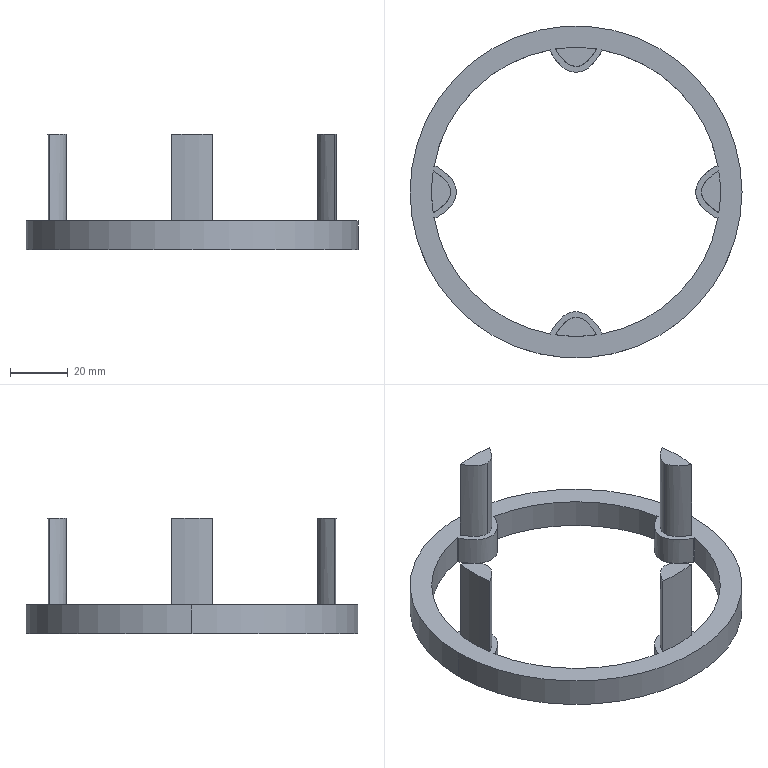Part | SolidWorks | features ICE 5, Extrusion 1, RefAxis 1, RefPoint 1 | 1 solid | 37 faces | box 115 x 115 x 40 mm | volume 37157 mm3 | plane 14 | spline 12 | cylinder 11 | commonest cylinder face diameters 100 x9 115 x2